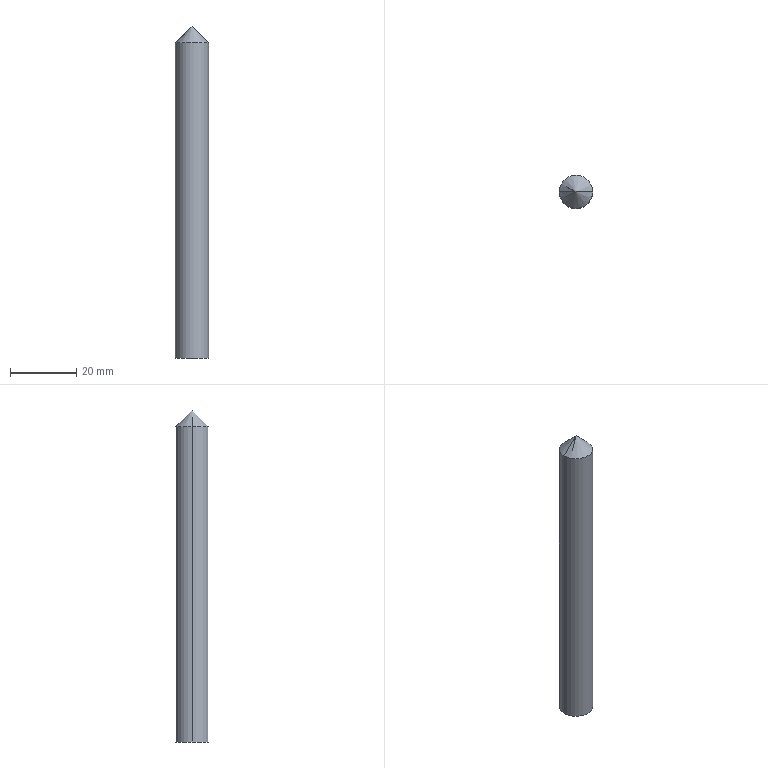Part | SolidWorks | features Chamfer 1, Extrusion 1 | 1 solid | 5 faces | box 10 x 10 x 100 mm | volume 7592 mm3 | cone 2 | cylinder 2 | plane 1 | commonest cylinder face diameters 10 x2
STEP:
#1=CARTESIAN_POINT('',(0.,0.,100.));
#2=VERTEX_POINT('',#1);
#3=CARTESIAN_POINT('',(-5.,0.,95.));
#4=VERTEX_POINT('',#3);
#5=CARTESIAN_POINT('',(-5.,0.,95.));
#6=DIRECTION('',(-0.7071,0.,-0.7071));
#7=VECTOR('',#6,1000.);
#8=LINE('',#5,#7);
#9=EDGE_CURVE('',#2,#4,#8,.T.);
#10=ORIENTED_EDGE('',*,*,#9,.F.);
#11=CARTESIAN_POINT('',(5.,0.,95.));
#12=VERTEX_POINT('',#11);
#13=CARTESIAN_POINT('',(5.,0.,95.));
#14=DIRECTION('',(0.7071,0.,-0.7071));
#15=VECTOR('',#14,1000.);
#16=LINE('',#13,#15);
#17=EDGE_CURVE('',#2,#12,#16,.T.);
#18=ORIENTED_EDGE('',*,*,#17,.T.);
#19=CARTESIAN_POINT('',(0.,0.,95.));
#20=DIRECTION('',(0.,0.,-1.));
#21=DIRECTION('',(1.,0.,0.));
#22=AXIS2_PLACEMENT_3D('',#19,#20,#21);
#23=CIRCLE('',#22,5.);
#24=EDGE_CURVE('',#4,#12,#23,.T.);
#25=ORIENTED_EDGE('',*,*,#24,.F.);
#26=EDGE_LOOP('',(#10,#18,#25));
#27=FACE_OUTER_BOUND('',#26,.T.);
#28=CARTESIAN_POINT('',(0.,0.,95.));
#29=DIRECTION('',(0.,0.,-1.));
#30=DIRECTION('',(-1.,0.,0.));
#31=AXIS2_PLACEMENT_3D('',#28,#29,#30);
#32=CONICAL_SURFACE('',#31,5.,0.7854);
#33=ADVANCED_FACE('',(#27),#32,.T.);
#34=ORIENTED_EDGE('',*,*,#24,.T.);
#35=CARTESIAN_POINT('',(5.,0.,0.));
#36=VERTEX_POINT('',#35);
#37=CARTESIAN_POINT('',(5.,0.,100.));
#38=DIRECTION('',(0.,0.,-1.));
#39=VECTOR('',#38,1000.);
#40=LINE('',#37,#39);
#41=EDGE_CURVE('',#12,#36,#40,.T.);
#42=ORIENTED_EDGE('',*,*,#41,.T.);
#43=CARTESIAN_POINT('',(-5.,0.,0.));
#44=VERTEX_POINT('',#43);
#45=CARTESIAN_POINT('',(0.,0.,0.));
#46=DIRECTION('',(0.,0.,1.));
#47=DIRECTION('',(1.,0.,0.));
#48=AXIS2_PLACEMENT_3D('',#45,#46,#47);
#49=CIRCLE('',#48,5.);
#50=EDGE_CURVE('',#36,#44,#49,.T.);
#51=ORIENTED_EDGE('',*,*,#50,.T.);
#52=CARTESIAN_POINT('',(-5.,0.,100.));
#53=DIRECTION('',(0.,0.,-1.));
#54=VECTOR('',#53,1000.);
#55=LINE('',#52,#54);
#56=EDGE_CURVE('',#4,#44,#55,.T.);
#57=ORIENTED_EDGE('',*,*,#56,.F.);
#58=EDGE_LOOP('',(#34,#42,#51,#57));
#59=FACE_OUTER_BOUND('',#58,.T.);
#60=CARTESIAN_POINT('',(0.,0.,100.));
#61=DIRECTION('',(0.,0.,-1.));
#62=DIRECTION('',(-1.,0.,0.));
#63=AXIS2_PLACEMENT_3D('',#60,#61,#62);
#64=CYLINDRICAL_SURFACE('',#63,5.);
#65=ADVANCED_FACE('',(#59),#64,.T.);
#66=ORIENTED_EDGE('',*,*,#41,.F.);
#67=CARTESIAN_POINT('',(0.,0.,95.));
#68=DIRECTION('',(0.,0.,-1.));
#69=DIRECTION('',(1.,0.,0.));
#70=AXIS2_PLACEMENT_3D('',#67,#68,#69);
#71=CIRCLE('',#70,5.);
#72=EDGE_CURVE('',#12,#4,#71,.T.);
#73=ORIENTED_EDGE('',*,*,#72,.T.);
#74=ORIENTED_EDGE('',*,*,#56,.T.);
#75=CARTESIAN_POINT('',(0.,0.,0.));
#76=DIRECTION('',(0.,0.,1.));
#77=DIRECTION('',(1.,0.,0.));
#78=AXIS2_PLACEMENT_3D('',#75,#76,#77);
#79=CIRCLE('',#78,5.);
#80=EDGE_CURVE('',#44,#36,#79,.T.);
#81=ORIENTED_EDGE('',*,*,#80,.T.);
#82=EDGE_LOOP('',(#66,#73,#74,#81));
#83=FACE_OUTER_BOUND('',#82,.T.);
#84=CARTESIAN_POINT('',(0.,0.,100.));
#85=DIRECTION('',(0.,0.,-1.));
#86=DIRECTION('',(-1.,0.,0.));
#87=AXIS2_PLACEMENT_3D('',#84,#85,#86);
#88=CYLINDRICAL_SURFACE('',#87,5.);
#89=ADVANCED_FACE('',(#83),#88,.T.);
#90=ORIENTED_EDGE('',*,*,#80,.F.);
#91=ORIENTED_EDGE('',*,*,#50,.F.);
#92=EDGE_LOOP('',(#90,#91));
#93=FACE_OUTER_BOUND('',#92,.T.);
#94=CARTESIAN_POINT('',(0.,0.,0.));
#95=DIRECTION('',(0.,0.,1.));
#96=DIRECTION('',(1.,0.,0.));
#97=AXIS2_PLACEMENT_3D('',#94,#95,#96);
#98=PLANE('',#97);
#99=ADVANCED_FACE('',(#93),#98,.F.);
#100=ORIENTED_EDGE('',*,*,#17,.F.);
#101=ORIENTED_EDGE('',*,*,#9,.T.);
#102=ORIENTED_EDGE('',*,*,#72,.F.);
#103=EDGE_LOOP('',(#100,#101,#102));
#104=FACE_OUTER_BOUND('',#103,.T.);
#105=CARTESIAN_POINT('',(0.,0.,95.));
#106=DIRECTION('',(0.,0.,-1.));
#107=DIRECTION('',(-1.,0.,0.));
#108=AXIS2_PLACEMENT_3D('',#105,#106,#107);
#109=CONICAL_SURFACE('',#108,5.,0.7854);
#110=ADVANCED_FACE('',(#104),#109,.T.);
#111=CLOSED_SHELL('',(#33,#65,#89,#99,#110));
#112=MANIFOLD_SOLID_BREP('',#111);
#113=CARTESIAN_POINT('',(0.,0.,0.));
#114=DIRECTION('',(0.,0.,1.));
#115=DIRECTION('',(1.,0.,0.));
#116=AXIS2_PLACEMENT_3D('',#113,#114,#115);
#117=(LENGTH_UNIT()NAMED_UNIT(*)SI_UNIT(.MILLI.,.METRE.));
#118=UNCERTAINTY_MEASURE_WITH_UNIT(LENGTH_MEASURE(0.00001),#117,'','');
#119=(NAMED_UNIT(*)PLANE_ANGLE_UNIT()SI_UNIT($,.RADIAN.));
#120=(NAMED_UNIT(*)SI_UNIT($,.STERADIAN.)SOLID_ANGLE_UNIT());
#121=(GEOMETRIC_REPRESENTATION_CONTEXT(3)GLOBAL_UNCERTAINTY_ASSIGNED_CONTEXT((#118))GLOBAL_UNIT_ASSIGNED_CONTEXT((#117,#119,#120))REPRESENTATION_CONTEXT('',''));
#122=ADVANCED_BREP_SHAPE_REPRESENTATION('',(#112,#116),#121);